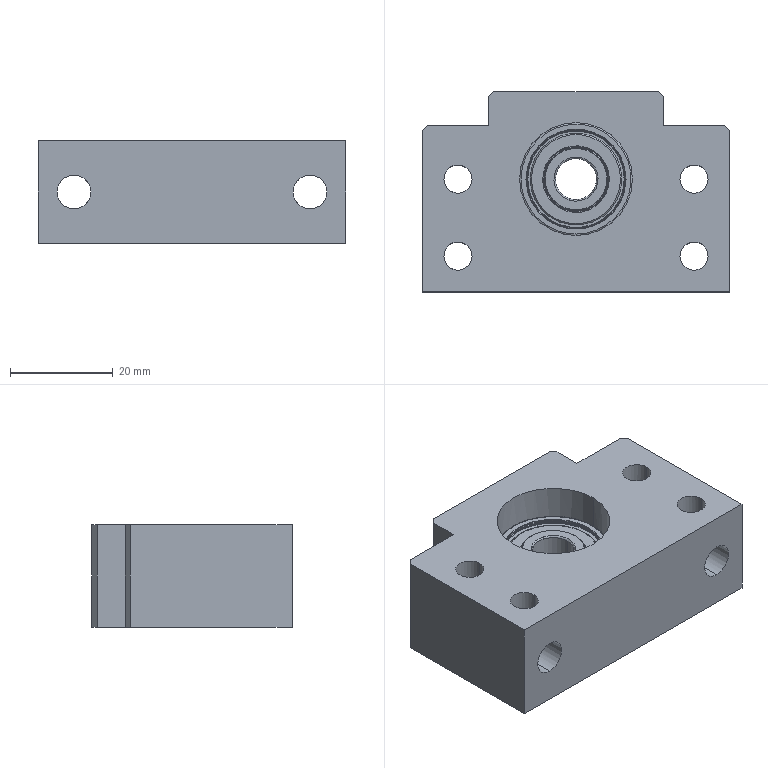Part | SolidWorks | features BaseBody 1 | 1 solid | 158 faces | box 60 x 39 x 20 mm | volume 33430 mm3 | cylinder 54 | cone 44 | torus 32 | plane 28 | commonest cylinder face diameters 5.5 x16 6.6 x4 11 x4 12.2 x4 12.6 x4 12.73 x4